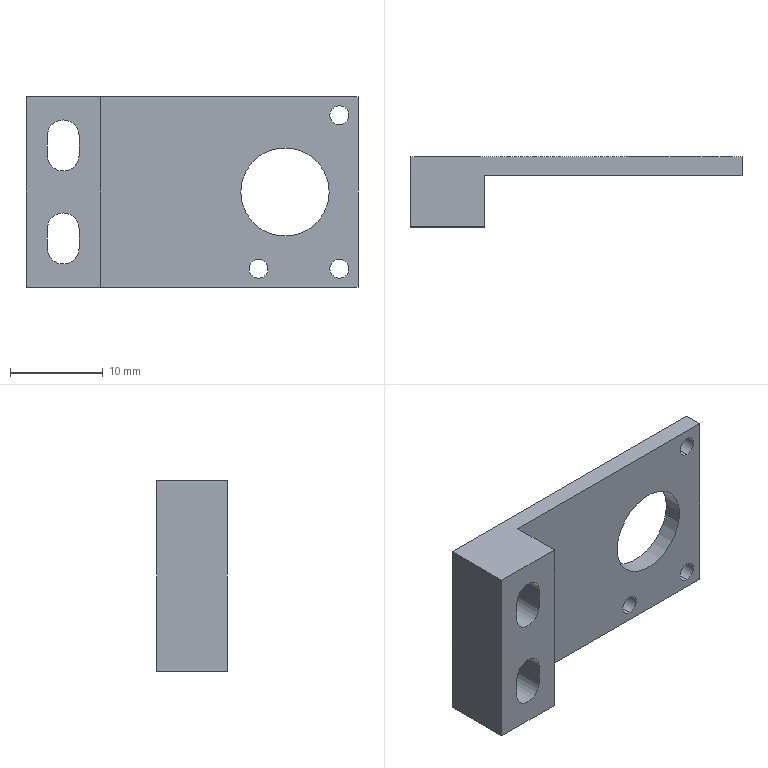Part | STEP file | 1 solid | 38 faces | box 35.7 x 7.55 x 20.5 mm | volume 1672 mm3 | cylinder 20 | plane 18 | commonest cylinder face diameters 2.05 x6 3.4 x6 7 x6 9.5 x2